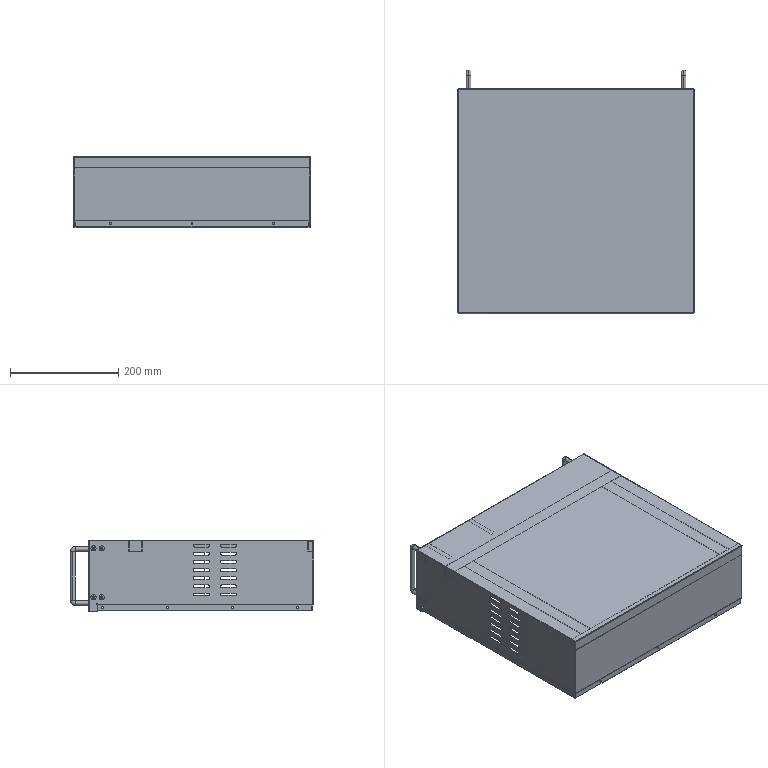Part | SolidWorks | features ICE 15, LPattern 7, SMBaseFlange 7, EdgeFlange 6, FlatPattern 6, SheetMetal 6, MirrorPattern 4, BossThin 3, CornerTrim 2, MirrorSolid 1, Split 1, Sweep 1 | 7 solids | 767 faces | box 437 x 449.5 x 132 mm | volume 626623 mm3 | plane 396 | cylinder 351 | spline 12 | torus 8 | commonest cylinder face diameters 5 x114 3.5 x48 0.2 x28 2.6 x28 4.5 x20 9.5 x20